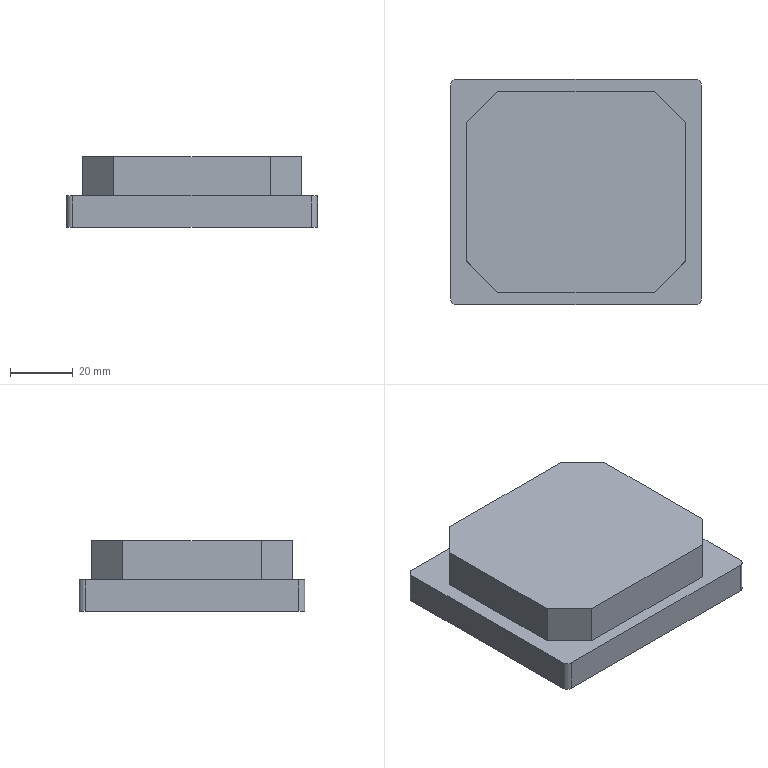Part | SolidWorks | features BaseBody 1 | 1 solid | 19 faces | box 80 x 72 x 22.5 mm | volume 111066 mm3 | plane 15 | cylinder 4 | commonest cylinder face diameters 4 x4
STEP:
#1=CARTESIAN_POINT('',(38.,-36.,0.));
#2=VERTEX_POINT('',#1);
#3=CARTESIAN_POINT('',(40.,-34.,0.));
#4=VERTEX_POINT('',#3);
#5=CARTESIAN_POINT('',(38.,-34.,0.));
#6=DIRECTION('',(0.,0.,1.));
#7=DIRECTION('',(-1.,0.,0.));
#8=AXIS2_PLACEMENT_3D('',#5,#6,#7);
#9=CIRCLE('',#8,2.);
#10=EDGE_CURVE('',#2,#4,#9,.T.);
#11=ORIENTED_EDGE('',*,*,#10,.F.);
#12=CARTESIAN_POINT('',(-38.,-36.,0.));
#13=VERTEX_POINT('',#12);
#14=CARTESIAN_POINT('',(-40.,-36.,0.));
#15=DIRECTION('',(1.,0.,0.));
#16=VECTOR('',#15,1000.);
#17=LINE('',#14,#16);
#18=EDGE_CURVE('',#13,#2,#17,.T.);
#19=ORIENTED_EDGE('',*,*,#18,.F.);
#20=CARTESIAN_POINT('',(-40.,-34.,0.));
#21=VERTEX_POINT('',#20);
#22=CARTESIAN_POINT('',(-38.,-34.,0.));
#23=DIRECTION('',(0.,0.,1.));
#24=DIRECTION('',(-1.,0.,0.));
#25=AXIS2_PLACEMENT_3D('',#22,#23,#24);
#26=CIRCLE('',#25,2.);
#27=EDGE_CURVE('',#21,#13,#26,.T.);
#28=ORIENTED_EDGE('',*,*,#27,.F.);
#29=CARTESIAN_POINT('',(-40.,34.,0.));
#30=VERTEX_POINT('',#29);
#31=CARTESIAN_POINT('',(-40.,-36.,0.));
#32=DIRECTION('',(0.,-1.,0.));
#33=VECTOR('',#32,1000.);
#34=LINE('',#31,#33);
#35=EDGE_CURVE('',#30,#21,#34,.T.);
#36=ORIENTED_EDGE('',*,*,#35,.F.);
#37=CARTESIAN_POINT('',(-38.,36.,0.));
#38=VERTEX_POINT('',#37);
#39=CARTESIAN_POINT('',(-38.,34.,0.));
#40=DIRECTION('',(0.,0.,1.));
#41=DIRECTION('',(-1.,0.,0.));
#42=AXIS2_PLACEMENT_3D('',#39,#40,#41);
#43=CIRCLE('',#42,2.);
#44=EDGE_CURVE('',#38,#30,#43,.T.);
#45=ORIENTED_EDGE('',*,*,#44,.F.);
#46=CARTESIAN_POINT('',(38.,36.,0.));
#47=VERTEX_POINT('',#46);
#48=CARTESIAN_POINT('',(-40.,36.,0.));
#49=DIRECTION('',(-1.,0.,0.));
#50=VECTOR('',#49,1000.);
#51=LINE('',#48,#50);
#52=EDGE_CURVE('',#47,#38,#51,.T.);
#53=ORIENTED_EDGE('',*,*,#52,.F.);
#54=CARTESIAN_POINT('',(40.,34.,0.));
#55=VERTEX_POINT('',#54);
#56=CARTESIAN_POINT('',(38.,34.,0.));
#57=DIRECTION('',(0.,0.,1.));
#58=DIRECTION('',(-1.,0.,0.));
#59=AXIS2_PLACEMENT_3D('',#56,#57,#58);
#60=CIRCLE('',#59,2.);
#61=EDGE_CURVE('',#55,#47,#60,.T.);
#62=ORIENTED_EDGE('',*,*,#61,.F.);
#63=CARTESIAN_POINT('',(40.,-36.,0.));
#64=DIRECTION('',(0.,1.,0.));
#65=VECTOR('',#64,1000.);
#66=LINE('',#63,#65);
#67=EDGE_CURVE('',#4,#55,#66,.T.);
#68=ORIENTED_EDGE('',*,*,#67,.F.);
#69=EDGE_LOOP('',(#11,#19,#28,#36,#45,#53,#62,#68));
#70=FACE_OUTER_BOUND('',#69,.T.);
#71=CARTESIAN_POINT('',(-40.,-36.,0.));
#72=DIRECTION('',(0.,0.,1.));
#73=DIRECTION('',(1.,0.,0.));
#74=AXIS2_PLACEMENT_3D('',#71,#72,#73);
#75=PLANE('',#74);
#76=ADVANCED_FACE('',(#70),#75,.F.);
#77=CARTESIAN_POINT('',(40.,-34.,10.));
#78=VERTEX_POINT('',#77);
#79=CARTESIAN_POINT('',(40.,-34.,10.));
#80=DIRECTION('',(0.,0.,1.));
#81=VECTOR('',#80,1000.);
#82=LINE('',#79,#81);
#83=EDGE_CURVE('',#4,#78,#82,.T.);
#84=ORIENTED_EDGE('',*,*,#83,.F.);
#85=ORIENTED_EDGE('',*,*,#67,.T.);
#86=CARTESIAN_POINT('',(40.,34.,10.));
#87=VERTEX_POINT('',#86);
#88=CARTESIAN_POINT('',(40.,34.,10.));
#89=DIRECTION('',(0.,0.,-1.));
#90=VECTOR('',#89,1000.);
#91=LINE('',#88,#90);
#92=EDGE_CURVE('',#87,#55,#91,.T.);
#93=ORIENTED_EDGE('',*,*,#92,.F.);
#94=CARTESIAN_POINT('',(40.,-36.,10.));
#95=DIRECTION('',(0.,1.,0.));
#96=VECTOR('',#95,1000.);
#97=LINE('',#94,#96);
#98=EDGE_CURVE('',#78,#87,#97,.T.);
#99=ORIENTED_EDGE('',*,*,#98,.F.);
#100=EDGE_LOOP('',(#84,#85,#93,#99));
#101=FACE_OUTER_BOUND('',#100,.T.);
#102=CARTESIAN_POINT('',(40.,-36.,10.));
#103=DIRECTION('',(-1.,0.,0.));
#104=DIRECTION('',(0.,0.,1.));
#105=AXIS2_PLACEMENT_3D('',#102,#103,#104);
#106=PLANE('',#105);
#107=ADVANCED_FACE('',(#101),#106,.F.);
#108=ORIENTED_EDGE('',*,*,#10,.T.);
#109=ORIENTED_EDGE('',*,*,#83,.T.);
#110=CARTESIAN_POINT('',(38.,-36.,10.));
#111=VERTEX_POINT('',#110);
#112=CARTESIAN_POINT('',(38.,-34.,10.));
#113=DIRECTION('',(0.,0.,-1.));
#114=DIRECTION('',(-1.,0.,0.));
#115=AXIS2_PLACEMENT_3D('',#112,#113,#114);
#116=CIRCLE('',#115,2.);
#117=EDGE_CURVE('',#78,#111,#116,.T.);
#118=ORIENTED_EDGE('',*,*,#117,.T.);
#119=CARTESIAN_POINT('',(38.,-36.,10.));
#120=DIRECTION('',(0.,0.,-1.));
#121=VECTOR('',#120,1000.);
#122=LINE('',#119,#121);
#123=EDGE_CURVE('',#111,#2,#122,.T.);
#124=ORIENTED_EDGE('',*,*,#123,.T.);
#125=EDGE_LOOP('',(#108,#109,#118,#124));
#126=FACE_OUTER_BOUND('',#125,.T.);
#127=CARTESIAN_POINT('',(38.,-34.,10.));
#128=DIRECTION('',(0.,0.,-1.));
#129=DIRECTION('',(-1.,0.,0.));
#130=AXIS2_PLACEMENT_3D('',#127,#128,#129);
#131=CYLINDRICAL_SURFACE('',#130,2.);
#132=ADVANCED_FACE('',(#126),#131,.T.);
#133=ORIENTED_EDGE('',*,*,#123,.F.);
#134=CARTESIAN_POINT('',(-38.,-36.,10.));
#135=VERTEX_POINT('',#134);
#136=CARTESIAN_POINT('',(-40.,-36.,10.));
#137=DIRECTION('',(1.,0.,0.));
#138=VECTOR('',#137,1000.);
#139=LINE('',#136,#138);
#140=EDGE_CURVE('',#135,#111,#139,.T.);
#141=ORIENTED_EDGE('',*,*,#140,.F.);
#142=CARTESIAN_POINT('',(-38.,-36.,10.));
#143=DIRECTION('',(0.,0.,1.));
#144=VECTOR('',#143,1000.);
#145=LINE('',#142,#144);
#146=EDGE_CURVE('',#13,#135,#145,.T.);
#147=ORIENTED_EDGE('',*,*,#146,.F.);
#148=ORIENTED_EDGE('',*,*,#18,.T.);
#149=EDGE_LOOP('',(#133,#141,#147,#148));
#150=FACE_OUTER_BOUND('',#149,.T.);
#151=CARTESIAN_POINT('',(-40.,-36.,10.));
#152=DIRECTION('',(0.,1.,0.));
#153=DIRECTION('',(0.,0.,1.));
#154=AXIS2_PLACEMENT_3D('',#151,#152,#153);
#155=PLANE('',#154);
#156=ADVANCED_FACE('',(#150),#155,.F.);
#157=ORIENTED_EDGE('',*,*,#27,.T.);
#158=ORIENTED_EDGE('',*,*,#146,.T.);
#159=CARTESIAN_POINT('',(-40.,-34.,10.));
#160=VERTEX_POINT('',#159);
#161=CARTESIAN_POINT('',(-38.,-34.,10.));
#162=DIRECTION('',(0.,0.,-1.));
#163=DIRECTION('',(-1.,0.,0.));
#164=AXIS2_PLACEMENT_3D('',#161,#162,#163);
#165=CIRCLE('',#164,2.);
#166=EDGE_CURVE('',#135,#160,#165,.T.);
#167=ORIENTED_EDGE('',*,*,#166,.T.);
#168=CARTESIAN_POINT('',(-40.,-34.,10.));
#169=DIRECTION('',(0.,0.,-1.));
#170=VECTOR('',#169,1000.);
#171=LINE('',#168,#170);
#172=EDGE_CURVE('',#160,#21,#171,.T.);
#173=ORIENTED_EDGE('',*,*,#172,.T.);
#174=EDGE_LOOP('',(#157,#158,#167,#173));
#175=FACE_OUTER_BOUND('',#174,.T.);
#176=CARTESIAN_POINT('',(-38.,-34.,10.));
#177=DIRECTION('',(0.,0.,-1.));
#178=DIRECTION('',(-1.,0.,0.));
#179=AXIS2_PLACEMENT_3D('',#176,#177,#178);
#180=CYLINDRICAL_SURFACE('',#179,2.);
#181=ADVANCED_FACE('',(#175),#180,.T.);
#182=CARTESIAN_POINT('',(-40.,34.,10.));
#183=VERTEX_POINT('',#182);
#184=CARTESIAN_POINT('',(-40.,34.,10.));
#185=DIRECTION('',(0.,0.,1.));
#186=VECTOR('',#185,1000.);
#187=LINE('',#184,#186);
#188=EDGE_CURVE('',#30,#183,#187,.T.);
#189=ORIENTED_EDGE('',*,*,#188,.F.);
#190=ORIENTED_EDGE('',*,*,#35,.T.);
#191=ORIENTED_EDGE('',*,*,#172,.F.);
#192=CARTESIAN_POINT('',(-40.,36.,10.));
#193=DIRECTION('',(0.,-1.,0.));
#194=VECTOR('',#193,1000.);
#195=LINE('',#192,#194);
#196=EDGE_CURVE('',#183,#160,#195,.T.);
#197=ORIENTED_EDGE('',*,*,#196,.F.);
#198=EDGE_LOOP('',(#189,#190,#191,#197));
#199=FACE_OUTER_BOUND('',#198,.T.);
#200=CARTESIAN_POINT('',(-40.,36.,10.));
#201=DIRECTION('',(1.,0.,0.));
#202=DIRECTION('',(0.,0.,-1.));
#203=AXIS2_PLACEMENT_3D('',#200,#201,#202);
#204=PLANE('',#203);
#205=ADVANCED_FACE('',(#199),#204,.F.);
#206=ORIENTED_EDGE('',*,*,#44,.T.);
#207=ORIENTED_EDGE('',*,*,#188,.T.);
#208=CARTESIAN_POINT('',(-38.,36.,10.));
#209=VERTEX_POINT('',#208);
#210=CARTESIAN_POINT('',(-38.,34.,10.));
#211=DIRECTION('',(0.,0.,-1.));
#212=DIRECTION('',(-1.,0.,0.));
#213=AXIS2_PLACEMENT_3D('',#210,#211,#212);
#214=CIRCLE('',#213,2.);
#215=EDGE_CURVE('',#183,#209,#214,.T.);
#216=ORIENTED_EDGE('',*,*,#215,.T.);
#217=CARTESIAN_POINT('',(-38.,36.,10.));
#218=DIRECTION('',(0.,0.,-1.));
#219=VECTOR('',#218,1000.);
#220=LINE('',#217,#219);
#221=EDGE_CURVE('',#209,#38,#220,.T.);
#222=ORIENTED_EDGE('',*,*,#221,.T.);
#223=EDGE_LOOP('',(#206,#207,#216,#222));
#224=FACE_OUTER_BOUND('',#223,.T.);
#225=CARTESIAN_POINT('',(-38.,34.,10.));
#226=DIRECTION('',(0.,0.,-1.));
#227=DIRECTION('',(-1.,0.,0.));
#228=AXIS2_PLACEMENT_3D('',#225,#226,#227);
#229=CYLINDRICAL_SURFACE('',#228,2.);
#230=ADVANCED_FACE('',(#224),#229,.T.);
#231=CARTESIAN_POINT('',(38.,36.,10.));
#232=VERTEX_POINT('',#231);
#233=CARTESIAN_POINT('',(38.,36.,10.));
#234=DIRECTION('',(0.,0.,1.));
#235=VECTOR('',#234,1000.);
#236=LINE('',#233,#235);
#237=EDGE_CURVE('',#47,#232,#236,.T.);
#238=ORIENTED_EDGE('',*,*,#237,.F.);
#239=ORIENTED_EDGE('',*,*,#52,.T.);
#240=ORIENTED_EDGE('',*,*,#221,.F.);
#241=CARTESIAN_POINT('',(40.,36.,10.));
#242=DIRECTION('',(-1.,0.,0.));
#243=VECTOR('',#242,1000.);
#244=LINE('',#241,#243);
#245=EDGE_CURVE('',#232,#209,#244,.T.);
#246=ORIENTED_EDGE('',*,*,#245,.F.);
#247=EDGE_LOOP('',(#238,#239,#240,#246));
#248=FACE_OUTER_BOUND('',#247,.T.);
#249=CARTESIAN_POINT('',(40.,36.,10.));
#250=DIRECTION('',(0.,-1.,0.));
#251=DIRECTION('',(0.,0.,-1.));
#252=AXIS2_PLACEMENT_3D('',#249,#250,#251);
#253=PLANE('',#252);
#254=ADVANCED_FACE('',(#248),#253,.F.);
#255=ORIENTED_EDGE('',*,*,#61,.T.);
#256=ORIENTED_EDGE('',*,*,#237,.T.);
#257=CARTESIAN_POINT('',(38.,34.,10.));
#258=DIRECTION('',(0.,0.,-1.));
#259=DIRECTION('',(-1.,0.,0.));
#260=AXIS2_PLACEMENT_3D('',#257,#258,#259);
#261=CIRCLE('',#260,2.);
#262=EDGE_CURVE('',#232,#87,#261,.T.);
#263=ORIENTED_EDGE('',*,*,#262,.T.);
#264=ORIENTED_EDGE('',*,*,#92,.T.);
#265=EDGE_LOOP('',(#255,#256,#263,#264));
#266=FACE_OUTER_BOUND('',#265,.T.);
#267=CARTESIAN_POINT('',(38.,34.,10.));
#268=DIRECTION('',(0.,0.,-1.));
#269=DIRECTION('',(-1.,0.,0.));
#270=AXIS2_PLACEMENT_3D('',#267,#268,#269);
#271=CYLINDRICAL_SURFACE('',#270,2.);
#272=ADVANCED_FACE('',(#266),#271,.T.);
#273=ORIENTED_EDGE('',*,*,#196,.T.);
#274=ORIENTED_EDGE('',*,*,#166,.F.);
#275=ORIENTED_EDGE('',*,*,#140,.T.);
#276=ORIENTED_EDGE('',*,*,#117,.F.);
#277=ORIENTED_EDGE('',*,*,#98,.T.);
#278=ORIENTED_EDGE('',*,*,#262,.F.);
#279=ORIENTED_EDGE('',*,*,#245,.T.);
#280=ORIENTED_EDGE('',*,*,#215,.F.);
#281=EDGE_LOOP('',(#273,#274,#275,#276,#277,#278,#279,#280));
#282=FACE_OUTER_BOUND('',#281,.T.);
#283=CARTESIAN_POINT('',(25.,-32.,10.));
#284=VERTEX_POINT('',#283);
#285=CARTESIAN_POINT('',(-25.,-32.,10.));
#286=VERTEX_POINT('',#285);
#287=CARTESIAN_POINT('',(-40.,-32.,10.));
#288=DIRECTION('',(-1.,0.,0.));
#289=VECTOR('',#288,1000.);
#290=LINE('',#287,#289);
#291=EDGE_CURVE('',#284,#286,#290,.T.);
#292=ORIENTED_EDGE('',*,*,#291,.T.);
#293=CARTESIAN_POINT('',(-35.,-22.,10.));
#294=VERTEX_POINT('',#293);
#295=CARTESIAN_POINT('',(-25.,-32.,10.));
#296=DIRECTION('',(-0.7071,0.7071,0.));
#297=VECTOR('',#296,1000.);
#298=LINE('',#295,#297);
#299=EDGE_CURVE('',#286,#294,#298,.T.);
#300=ORIENTED_EDGE('',*,*,#299,.T.);
#301=CARTESIAN_POINT('',(-35.,22.,10.));
#302=VERTEX_POINT('',#301);
#303=CARTESIAN_POINT('',(-35.,-36.,10.));
#304=DIRECTION('',(0.,1.,0.));
#305=VECTOR('',#304,1000.);
#306=LINE('',#303,#305);
#307=EDGE_CURVE('',#294,#302,#306,.T.);
#308=ORIENTED_EDGE('',*,*,#307,.T.);
#309=CARTESIAN_POINT('',(-25.,32.,10.));
#310=VERTEX_POINT('',#309);
#311=CARTESIAN_POINT('',(-35.,22.,10.));
#312=DIRECTION('',(0.7071,0.7071,0.));
#313=VECTOR('',#312,1000.);
#314=LINE('',#311,#313);
#315=EDGE_CURVE('',#302,#310,#314,.T.);
#316=ORIENTED_EDGE('',*,*,#315,.T.);
#317=CARTESIAN_POINT('',(25.,32.,10.));
#318=VERTEX_POINT('',#317);
#319=CARTESIAN_POINT('',(-40.,32.,10.));
#320=DIRECTION('',(1.,0.,0.));
#321=VECTOR('',#320,1000.);
#322=LINE('',#319,#321);
#323=EDGE_CURVE('',#310,#318,#322,.T.);
#324=ORIENTED_EDGE('',*,*,#323,.T.);
#325=CARTESIAN_POINT('',(35.,22.,10.));
#326=VERTEX_POINT('',#325);
#327=CARTESIAN_POINT('',(25.,32.,10.));
#328=DIRECTION('',(0.7071,-0.7071,0.));
#329=VECTOR('',#328,1000.);
#330=LINE('',#327,#329);
#331=EDGE_CURVE('',#318,#326,#330,.T.);
#332=ORIENTED_EDGE('',*,*,#331,.T.);
#333=CARTESIAN_POINT('',(35.,-22.,10.));
#334=VERTEX_POINT('',#333);
#335=CARTESIAN_POINT('',(35.,-36.,10.));
#336=DIRECTION('',(0.,-1.,0.));
#337=VECTOR('',#336,1000.);
#338=LINE('',#335,#337);
#339=EDGE_CURVE('',#326,#334,#338,.T.);
#340=ORIENTED_EDGE('',*,*,#339,.T.);
#341=CARTESIAN_POINT('',(35.,-22.,10.));
#342=DIRECTION('',(-0.7071,-0.7071,0.));
#343=VECTOR('',#342,1000.);
#344=LINE('',#341,#343);
#345=EDGE_CURVE('',#334,#284,#344,.T.);
#346=ORIENTED_EDGE('',*,*,#345,.T.);
#347=EDGE_LOOP('',(#292,#300,#308,#316,#324,#332,#340,#346));
#348=FACE_BOUND('',#347,.T.);
#349=CARTESIAN_POINT('',(-40.,-36.,10.));
#350=DIRECTION('',(0.,0.,1.));
#351=DIRECTION('',(1.,0.,0.));
#352=AXIS2_PLACEMENT_3D('',#349,#350,#351);
#353=PLANE('',#352);
#354=ADVANCED_FACE('',(#282,#348),#353,.T.);
#355=CARTESIAN_POINT('',(-35.,-22.,22.5));
#356=VERTEX_POINT('',#355);
#357=CARTESIAN_POINT('',(-35.,-22.,22.5));
#358=DIRECTION('',(0.,0.,1.));
#359=VECTOR('',#358,1000.);
#360=LINE('',#357,#359);
#361=EDGE_CURVE('',#294,#356,#360,.T.);
#362=ORIENTED_EDGE('',*,*,#361,.F.);
#363=ORIENTED_EDGE('',*,*,#299,.F.);
#364=CARTESIAN_POINT('',(-25.,-32.,22.5));
#365=VERTEX_POINT('',#364);
#366=CARTESIAN_POINT('',(-25.,-32.,22.5));
#367=DIRECTION('',(0.,0.,-1.));
#368=VECTOR('',#367,1000.);
#369=LINE('',#366,#368);
#370=EDGE_CURVE('',#365,#286,#369,.T.);
#371=ORIENTED_EDGE('',*,*,#370,.F.);
#372=CARTESIAN_POINT('',(-25.,-32.,22.5));
#373=DIRECTION('',(0.7071,-0.7071,0.));
#374=VECTOR('',#373,1000.);
#375=LINE('',#372,#374);
#376=EDGE_CURVE('',#356,#365,#375,.T.);
#377=ORIENTED_EDGE('',*,*,#376,.F.);
#378=EDGE_LOOP('',(#362,#363,#371,#377));
#379=FACE_OUTER_BOUND('',#378,.T.);
#380=CARTESIAN_POINT('',(-25.,-32.,22.5));
#381=DIRECTION('',(0.7071,0.7071,0.));
#382=DIRECTION('',(-0.7071,0.7071,0.));
#383=AXIS2_PLACEMENT_3D('',#380,#381,#382);
#384=PLANE('',#383);
#385=ADVANCED_FACE('',(#379),#384,.F.);
#386=CARTESIAN_POINT('',(25.,-32.,22.5));
#387=VERTEX_POINT('',#386);
#388=CARTESIAN_POINT('',(25.,-32.,22.5));
#389=DIRECTION('',(0.,0.,-1.));
#390=VECTOR('',#389,1000.);
#391=LINE('',#388,#390);
#392=EDGE_CURVE('',#387,#284,#391,.T.);
#393=ORIENTED_EDGE('',*,*,#392,.F.);
#394=CARTESIAN_POINT('',(-35.,-32.,22.5));
#395=DIRECTION('',(1.,0.,0.));
#396=VECTOR('',#395,1000.);
#397=LINE('',#394,#396);
#398=EDGE_CURVE('',#365,#387,#397,.T.);
#399=ORIENTED_EDGE('',*,*,#398,.F.);
#400=ORIENTED_EDGE('',*,*,#370,.T.);
#401=ORIENTED_EDGE('',*,*,#291,.F.);
#402=EDGE_LOOP('',(#393,#399,#400,#401));
#403=FACE_OUTER_BOUND('',#402,.T.);
#404=CARTESIAN_POINT('',(-35.,-32.,22.5));
#405=DIRECTION('',(0.,1.,0.));
#406=DIRECTION('',(0.,0.,1.));
#407=AXIS2_PLACEMENT_3D('',#404,#405,#406);
#408=PLANE('',#407);
#409=ADVANCED_FACE('',(#403),#408,.F.);
#410=ORIENTED_EDGE('',*,*,#392,.T.);
#411=ORIENTED_EDGE('',*,*,#345,.F.);
#412=CARTESIAN_POINT('',(35.,-22.,22.5));
#413=VERTEX_POINT('',#412);
#414=CARTESIAN_POINT('',(35.,-22.,22.5));
#415=DIRECTION('',(0.,0.,-1.));
#416=VECTOR('',#415,1000.);
#417=LINE('',#414,#416);
#418=EDGE_CURVE('',#413,#334,#417,.T.);
#419=ORIENTED_EDGE('',*,*,#418,.F.);
#420=CARTESIAN_POINT('',(35.,-22.,22.5));
#421=DIRECTION('',(0.7071,0.7071,0.));
#422=VECTOR('',#421,1000.);
#423=LINE('',#420,#422);
#424=EDGE_CURVE('',#387,#413,#423,.T.);
#425=ORIENTED_EDGE('',*,*,#424,.F.);
#426=EDGE_LOOP('',(#410,#411,#419,#425));
#427=FACE_OUTER_BOUND('',#426,.T.);
#428=CARTESIAN_POINT('',(35.,-22.,22.5));
#429=DIRECTION('',(-0.7071,0.7071,0.));
#430=DIRECTION('',(-0.7071,-0.7071,0.));
#431=AXIS2_PLACEMENT_3D('',#428,#429,#430);
#432=PLANE('',#431);
#433=ADVANCED_FACE('',(#427),#432,.F.);
#434=ORIENTED_EDGE('',*,*,#418,.T.);
#435=ORIENTED_EDGE('',*,*,#339,.F.);
#436=CARTESIAN_POINT('',(35.,22.,22.5));
#437=VERTEX_POINT('',#436);
#438=CARTESIAN_POINT('',(35.,22.,22.5));
#439=DIRECTION('',(0.,0.,-1.));
#440=VECTOR('',#439,1000.);
#441=LINE('',#438,#440);
#442=EDGE_CURVE('',#437,#326,#441,.T.);
#443=ORIENTED_EDGE('',*,*,#442,.F.);
#444=CARTESIAN_POINT('',(35.,-32.,22.5));
#445=DIRECTION('',(0.,1.,0.));
#446=VECTOR('',#445,1000.);
#447=LINE('',#444,#446);
#448=EDGE_CURVE('',#413,#437,#447,.T.);
#449=ORIENTED_EDGE('',*,*,#448,.F.);
#450=EDGE_LOOP('',(#434,#435,#443,#449));
#451=FACE_OUTER_BOUND('',#450,.T.);
#452=CARTESIAN_POINT('',(35.,-32.,22.5));
#453=DIRECTION('',(-1.,0.,0.));
#454=DIRECTION('',(0.,0.,1.));
#455=AXIS2_PLACEMENT_3D('',#452,#453,#454);
#456=PLANE('',#455);
#457=ADVANCED_FACE('',(#451),#456,.F.);
#458=ORIENTED_EDGE('',*,*,#442,.T.);
#459=ORIENTED_EDGE('',*,*,#331,.F.);
#460=CARTESIAN_POINT('',(25.,32.,22.5));
#461=VERTEX_POINT('',#460);
#462=CARTESIAN_POINT('',(25.,32.,22.5));
#463=DIRECTION('',(0.,0.,-1.));
#464=VECTOR('',#463,1000.);
#465=LINE('',#462,#464);
#466=EDGE_CURVE('',#461,#318,#465,.T.);
#467=ORIENTED_EDGE('',*,*,#466,.F.);
#468=CARTESIAN_POINT('',(25.,32.,22.5));
#469=DIRECTION('',(-0.7071,0.7071,0.));
#470=VECTOR('',#469,1000.);
#471=LINE('',#468,#470);
#472=EDGE_CURVE('',#437,#461,#471,.T.);
#473=ORIENTED_EDGE('',*,*,#472,.F.);
#474=EDGE_LOOP('',(#458,#459,#467,#473));
#475=FACE_OUTER_BOUND('',#474,.T.);
#476=CARTESIAN_POINT('',(25.,32.,22.5));
#477=DIRECTION('',(-0.7071,-0.7071,0.));
#478=DIRECTION('',(0.7071,-0.7071,0.));
#479=AXIS2_PLACEMENT_3D('',#476,#477,#478);
#480=PLANE('',#479);
#481=ADVANCED_FACE('',(#475),#480,.F.);
#482=CARTESIAN_POINT('',(-25.,32.,22.5));
#483=VERTEX_POINT('',#482);
#484=CARTESIAN_POINT('',(-25.,32.,22.5));
#485=DIRECTION('',(0.,0.,-1.));
#486=VECTOR('',#485,1000.);
#487=LINE('',#484,#486);
#488=EDGE_CURVE('',#483,#310,#487,.T.);
#489=ORIENTED_EDGE('',*,*,#488,.F.);
#490=CARTESIAN_POINT('',(35.,32.,22.5));
#491=DIRECTION('',(-1.,0.,0.));
#492=VECTOR('',#491,1000.);
#493=LINE('',#490,#492);
#494=EDGE_CURVE('',#461,#483,#493,.T.);
#495=ORIENTED_EDGE('',*,*,#494,.F.);
#496=ORIENTED_EDGE('',*,*,#466,.T.);
#497=ORIENTED_EDGE('',*,*,#323,.F.);
#498=EDGE_LOOP('',(#489,#495,#496,#497));
#499=FACE_OUTER_BOUND('',#498,.T.);
#500=CARTESIAN_POINT('',(35.,32.,22.5));
#501=DIRECTION('',(0.,-1.,0.));
#502=DIRECTION('',(0.,0.,-1.));
#503=AXIS2_PLACEMENT_3D('',#500,#501,#502);
#504=PLANE('',#503);
#505=ADVANCED_FACE('',(#499),#504,.F.);
#506=ORIENTED_EDGE('',*,*,#488,.T.);
#507=ORIENTED_EDGE('',*,*,#315,.F.);
#508=CARTESIAN_POINT('',(-35.,22.,22.5));
#509=VERTEX_POINT('',#508);
#510=CARTESIAN_POINT('',(-35.,22.,22.5));
#511=DIRECTION('',(0.,0.,-1.));
#512=VECTOR('',#511,1000.);
#513=LINE('',#510,#512);
#514=EDGE_CURVE('',#509,#302,#513,.T.);
#515=ORIENTED_EDGE('',*,*,#514,.F.);
#516=CARTESIAN_POINT('',(-35.,22.,22.5));
#517=DIRECTION('',(-0.7071,-0.7071,0.));
#518=VECTOR('',#517,1000.);
#519=LINE('',#516,#518);
#520=EDGE_CURVE('',#483,#509,#519,.T.);
#521=ORIENTED_EDGE('',*,*,#520,.F.);
#522=EDGE_LOOP('',(#506,#507,#515,#521));
#523=FACE_OUTER_BOUND('',#522,.T.);
#524=CARTESIAN_POINT('',(-35.,22.,22.5));
#525=DIRECTION('',(0.7071,-0.7071,0.));
#526=DIRECTION('',(0.7071,0.7071,0.));
#527=AXIS2_PLACEMENT_3D('',#524,#525,#526);
#528=PLANE('',#527);
#529=ADVANCED_FACE('',(#523),#528,.F.);
#530=ORIENTED_EDGE('',*,*,#361,.T.);
#531=CARTESIAN_POINT('',(-35.,32.,22.5));
#532=DIRECTION('',(0.,-1.,0.));
#533=VECTOR('',#532,1000.);
#534=LINE('',#531,#533);
#535=EDGE_CURVE('',#509,#356,#534,.T.);
#536=ORIENTED_EDGE('',*,*,#535,.F.);
#537=ORIENTED_EDGE('',*,*,#514,.T.);
#538=ORIENTED_EDGE('',*,*,#307,.F.);
#539=EDGE_LOOP('',(#530,#536,#537,#538));
#540=FACE_OUTER_BOUND('',#539,.T.);
#541=CARTESIAN_POINT('',(-35.,32.,22.5));
#542=DIRECTION('',(1.,0.,0.));
#543=DIRECTION('',(0.,0.,-1.));
#544=AXIS2_PLACEMENT_3D('',#541,#542,#543);
#545=PLANE('',#544);
#546=ADVANCED_FACE('',(#540),#545,.F.);
#547=ORIENTED_EDGE('',*,*,#535,.T.);
#548=ORIENTED_EDGE('',*,*,#376,.T.);
#549=ORIENTED_EDGE('',*,*,#398,.T.);
#550=ORIENTED_EDGE('',*,*,#424,.T.);
#551=ORIENTED_EDGE('',*,*,#448,.T.);
#552=ORIENTED_EDGE('',*,*,#472,.T.);
#553=ORIENTED_EDGE('',*,*,#494,.T.);
#554=ORIENTED_EDGE('',*,*,#520,.T.);
#555=EDGE_LOOP('',(#547,#548,#549,#550,#551,#552,#553,#554));
#556=FACE_OUTER_BOUND('',#555,.T.);
#557=CARTESIAN_POINT('',(-35.,-32.,22.5));
#558=DIRECTION('',(0.,0.,1.));
#559=DIRECTION('',(1.,0.,0.));
#560=AXIS2_PLACEMENT_3D('',#557,#558,#559);
#561=PLANE('',#560);
#562=ADVANCED_FACE('',(#556),#561,.T.);
#563=CLOSED_SHELL('',(#76,#107,#132,#156,#181,#205,#230,#254,#272,#354,#385,#409,#433,#457,#481,#505,#529,#546,#562));
#564=MANIFOLD_SOLID_BREP('',#563);
#565=CARTESIAN_POINT('',(0.,0.,0.));
#566=DIRECTION('',(0.,0.,1.));
#567=DIRECTION('',(1.,0.,0.));
#568=AXIS2_PLACEMENT_3D('',#565,#566,#567);
#569=(LENGTH_UNIT()NAMED_UNIT(*)SI_UNIT(.MILLI.,.METRE.));
#570=UNCERTAINTY_MEASURE_WITH_UNIT(LENGTH_MEASURE(0.00001),#569,'','');
#571=(NAMED_UNIT(*)PLANE_ANGLE_UNIT()SI_UNIT($,.RADIAN.));
#572=(NAMED_UNIT(*)SI_UNIT($,.STERADIAN.)SOLID_ANGLE_UNIT());
#573=(GEOMETRIC_REPRESENTATION_CONTEXT(3)GLOBAL_UNCERTAINTY_ASSIGNED_CONTEXT((#570))GLOBAL_UNIT_ASSIGNED_CONTEXT((#569,#571,#572))REPRESENTATION_CONTEXT('',''));
#574=ADVANCED_BREP_SHAPE_REPRESENTATION('',(#564,#568),#573);